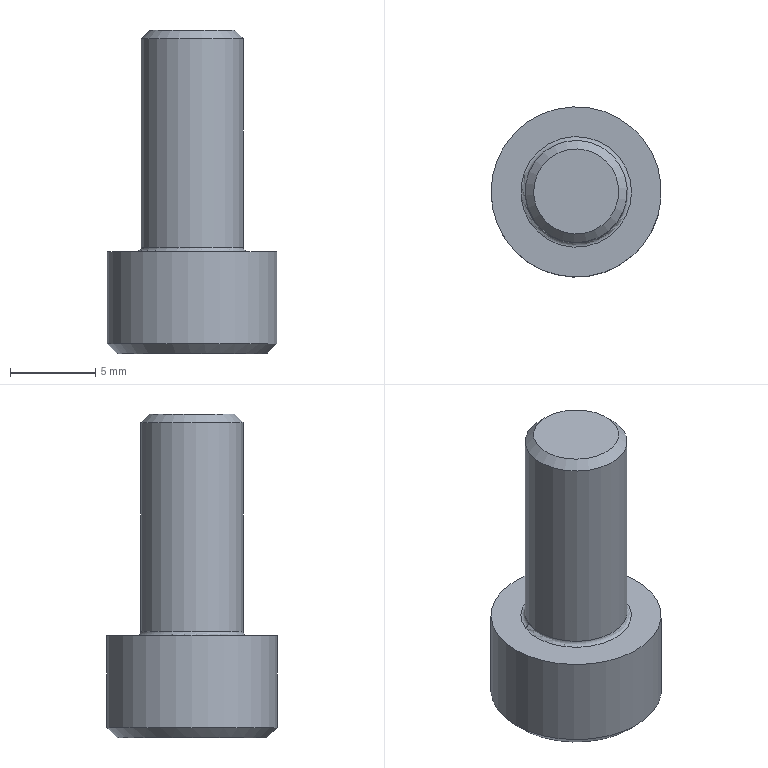Part | STEP file | solid 209 | 1 solid | 21 faces | box 10 x 10 x 19 mm | volume 766.17 mm3 | plane 10 | sphere 6 | cylinder 2 | cone 2 | torus 1 | commonest cylinder face diameters 6 x1 10 x1